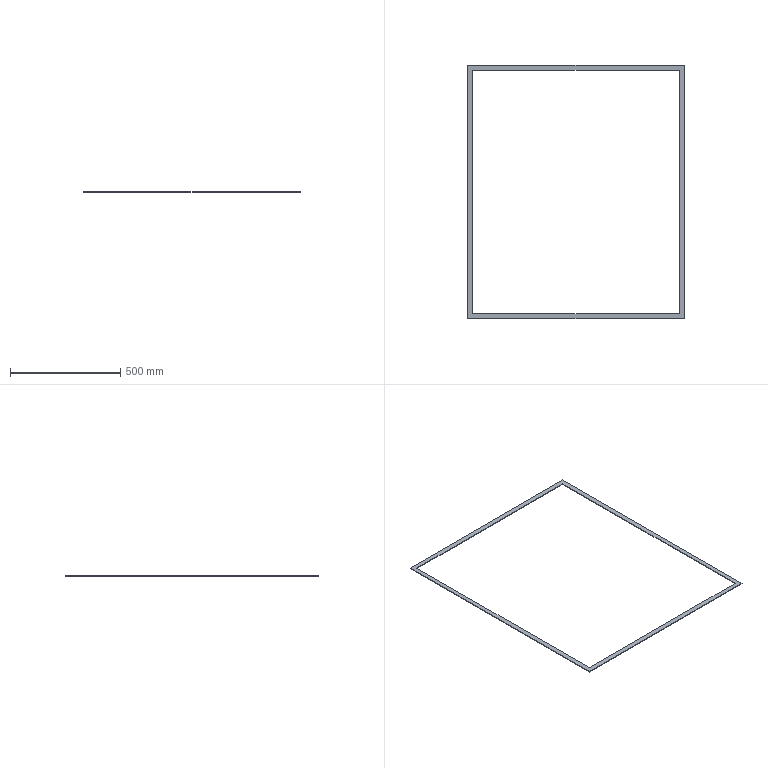Part | STEP file | 750038384 | 1 solid | 10 faces | box 981 x 1150 x 3 mm | volume 275484 mm3 | plane 10
STEP:
#1=CARTESIAN_POINT('',(490.5,-575.,0.));
#2=VERTEX_POINT('',#1);
#3=CARTESIAN_POINT('',(490.5,575.,0.));
#4=VERTEX_POINT('',#3);
#5=CARTESIAN_POINT('',(490.5,0.,0.));
#6=DIRECTION('',(0.,1.,0.));
#7=VECTOR('',#6,1000.);
#8=LINE('',#5,#7);
#9=EDGE_CURVE('',#2,#4,#8,.T.);
#10=ORIENTED_EDGE('',*,*,#9,.F.);
#11=CARTESIAN_POINT('',(-490.5,-575.,0.));
#12=VERTEX_POINT('',#11);
#13=CARTESIAN_POINT('',(0.,-575.,0.));
#14=DIRECTION('',(1.,0.,0.));
#15=VECTOR('',#14,1000.);
#16=LINE('',#13,#15);
#17=EDGE_CURVE('',#12,#2,#16,.T.);
#18=ORIENTED_EDGE('',*,*,#17,.F.);
#19=CARTESIAN_POINT('',(-490.5,575.,0.));
#20=VERTEX_POINT('',#19);
#21=CARTESIAN_POINT('',(-490.5,0.,0.));
#22=DIRECTION('',(0.,-1.,0.));
#23=VECTOR('',#22,1000.);
#24=LINE('',#21,#23);
#25=EDGE_CURVE('',#20,#12,#24,.T.);
#26=ORIENTED_EDGE('',*,*,#25,.F.);
#27=CARTESIAN_POINT('',(0.,575.,0.));
#28=DIRECTION('',(-1.,0.,0.));
#29=VECTOR('',#28,1000.);
#30=LINE('',#27,#29);
#31=EDGE_CURVE('',#4,#20,#30,.T.);
#32=ORIENTED_EDGE('',*,*,#31,.F.);
#33=EDGE_LOOP('',(#10,#18,#26,#32));
#34=FACE_OUTER_BOUND('',#33,.T.);
#35=CARTESIAN_POINT('',(468.5,-553.,0.));
#36=VERTEX_POINT('',#35);
#37=CARTESIAN_POINT('',(-468.5,-553.,0.));
#38=VERTEX_POINT('',#37);
#39=CARTESIAN_POINT('',(0.,-553.,0.));
#40=DIRECTION('',(-1.,0.,0.));
#41=VECTOR('',#40,1000.);
#42=LINE('',#39,#41);
#43=EDGE_CURVE('',#36,#38,#42,.T.);
#44=ORIENTED_EDGE('',*,*,#43,.F.);
#45=CARTESIAN_POINT('',(468.5,553.,0.));
#46=VERTEX_POINT('',#45);
#47=CARTESIAN_POINT('',(468.5,0.,0.));
#48=DIRECTION('',(0.,-1.,0.));
#49=VECTOR('',#48,1000.);
#50=LINE('',#47,#49);
#51=EDGE_CURVE('',#46,#36,#50,.T.);
#52=ORIENTED_EDGE('',*,*,#51,.F.);
#53=CARTESIAN_POINT('',(-468.5,553.,0.));
#54=VERTEX_POINT('',#53);
#55=CARTESIAN_POINT('',(0.,553.,0.));
#56=DIRECTION('',(1.,0.,0.));
#57=VECTOR('',#56,1000.);
#58=LINE('',#55,#57);
#59=EDGE_CURVE('',#54,#46,#58,.T.);
#60=ORIENTED_EDGE('',*,*,#59,.F.);
#61=CARTESIAN_POINT('',(-468.5,0.,0.));
#62=DIRECTION('',(0.,1.,0.));
#63=VECTOR('',#62,1000.);
#64=LINE('',#61,#63);
#65=EDGE_CURVE('',#38,#54,#64,.T.);
#66=ORIENTED_EDGE('',*,*,#65,.F.);
#67=EDGE_LOOP('',(#44,#52,#60,#66));
#68=FACE_BOUND('',#67,.T.);
#69=CARTESIAN_POINT('',(0.,0.,0.));
#70=DIRECTION('',(0.,0.,1.));
#71=DIRECTION('',(1.,0.,0.));
#72=AXIS2_PLACEMENT_3D('',#69,#70,#71);
#73=PLANE('',#72);
#74=ADVANCED_FACE('',(#34,#68),#73,.F.);
#75=CARTESIAN_POINT('',(-490.5,575.,3.));
#76=VERTEX_POINT('',#75);
#77=CARTESIAN_POINT('',(-490.5,575.,3.));
#78=DIRECTION('',(0.,0.,-1.));
#79=VECTOR('',#78,1000.);
#80=LINE('',#77,#79);
#81=EDGE_CURVE('',#76,#20,#80,.T.);
#82=ORIENTED_EDGE('',*,*,#81,.F.);
#83=CARTESIAN_POINT('',(490.5,575.,3.));
#84=VERTEX_POINT('',#83);
#85=CARTESIAN_POINT('',(490.5,575.,3.));
#86=DIRECTION('',(-1.,0.,0.));
#87=VECTOR('',#86,1000.);
#88=LINE('',#85,#87);
#89=EDGE_CURVE('',#84,#76,#88,.T.);
#90=ORIENTED_EDGE('',*,*,#89,.F.);
#91=CARTESIAN_POINT('',(490.5,575.,3.));
#92=DIRECTION('',(0.,0.,1.));
#93=VECTOR('',#92,1000.);
#94=LINE('',#91,#93);
#95=EDGE_CURVE('',#4,#84,#94,.T.);
#96=ORIENTED_EDGE('',*,*,#95,.F.);
#97=ORIENTED_EDGE('',*,*,#31,.T.);
#98=EDGE_LOOP('',(#82,#90,#96,#97));
#99=FACE_OUTER_BOUND('',#98,.T.);
#100=CARTESIAN_POINT('',(490.5,575.,3.));
#101=DIRECTION('',(0.,-1.,0.));
#102=DIRECTION('',(0.,0.,-1.));
#103=AXIS2_PLACEMENT_3D('',#100,#101,#102);
#104=PLANE('',#103);
#105=ADVANCED_FACE('',(#99),#104,.F.);
#106=ORIENTED_EDGE('',*,*,#95,.T.);
#107=CARTESIAN_POINT('',(490.5,-575.,3.));
#108=VERTEX_POINT('',#107);
#109=CARTESIAN_POINT('',(490.5,-575.,3.));
#110=DIRECTION('',(0.,1.,0.));
#111=VECTOR('',#110,1000.);
#112=LINE('',#109,#111);
#113=EDGE_CURVE('',#108,#84,#112,.T.);
#114=ORIENTED_EDGE('',*,*,#113,.F.);
#115=CARTESIAN_POINT('',(490.5,-575.,3.));
#116=DIRECTION('',(0.,0.,1.));
#117=VECTOR('',#116,1000.);
#118=LINE('',#115,#117);
#119=EDGE_CURVE('',#2,#108,#118,.T.);
#120=ORIENTED_EDGE('',*,*,#119,.F.);
#121=ORIENTED_EDGE('',*,*,#9,.T.);
#122=EDGE_LOOP('',(#106,#114,#120,#121));
#123=FACE_OUTER_BOUND('',#122,.T.);
#124=CARTESIAN_POINT('',(490.5,-575.,3.));
#125=DIRECTION('',(-1.,0.,0.));
#126=DIRECTION('',(0.,-1.,0.));
#127=AXIS2_PLACEMENT_3D('',#124,#125,#126);
#128=PLANE('',#127);
#129=ADVANCED_FACE('',(#123),#128,.F.);
#130=ORIENTED_EDGE('',*,*,#119,.T.);
#131=CARTESIAN_POINT('',(-490.5,-575.,3.));
#132=VERTEX_POINT('',#131);
#133=CARTESIAN_POINT('',(-490.5,-575.,3.));
#134=DIRECTION('',(1.,0.,0.));
#135=VECTOR('',#134,1000.);
#136=LINE('',#133,#135);
#137=EDGE_CURVE('',#132,#108,#136,.T.);
#138=ORIENTED_EDGE('',*,*,#137,.F.);
#139=CARTESIAN_POINT('',(-490.5,-575.,3.));
#140=DIRECTION('',(0.,0.,1.));
#141=VECTOR('',#140,1000.);
#142=LINE('',#139,#141);
#143=EDGE_CURVE('',#12,#132,#142,.T.);
#144=ORIENTED_EDGE('',*,*,#143,.F.);
#145=ORIENTED_EDGE('',*,*,#17,.T.);
#146=EDGE_LOOP('',(#130,#138,#144,#145));
#147=FACE_OUTER_BOUND('',#146,.T.);
#148=CARTESIAN_POINT('',(-490.5,-575.,3.));
#149=DIRECTION('',(0.,1.,0.));
#150=DIRECTION('',(0.,0.,1.));
#151=AXIS2_PLACEMENT_3D('',#148,#149,#150);
#152=PLANE('',#151);
#153=ADVANCED_FACE('',(#147),#152,.F.);
#154=ORIENTED_EDGE('',*,*,#143,.T.);
#155=CARTESIAN_POINT('',(-490.5,575.,3.));
#156=DIRECTION('',(0.,-1.,0.));
#157=VECTOR('',#156,1000.);
#158=LINE('',#155,#157);
#159=EDGE_CURVE('',#76,#132,#158,.T.);
#160=ORIENTED_EDGE('',*,*,#159,.F.);
#161=ORIENTED_EDGE('',*,*,#81,.T.);
#162=ORIENTED_EDGE('',*,*,#25,.T.);
#163=EDGE_LOOP('',(#154,#160,#161,#162));
#164=FACE_OUTER_BOUND('',#163,.T.);
#165=CARTESIAN_POINT('',(-490.5,575.,3.));
#166=DIRECTION('',(1.,0.,0.));
#167=DIRECTION('',(0.,1.,0.));
#168=AXIS2_PLACEMENT_3D('',#165,#166,#167);
#169=PLANE('',#168);
#170=ADVANCED_FACE('',(#164),#169,.F.);
#171=CARTESIAN_POINT('',(-468.5,553.,3.));
#172=VERTEX_POINT('',#171);
#173=CARTESIAN_POINT('',(-468.5,-553.,3.));
#174=VERTEX_POINT('',#173);
#175=CARTESIAN_POINT('',(-468.5,553.,3.));
#176=DIRECTION('',(0.,-1.,0.));
#177=VECTOR('',#176,1000.);
#178=LINE('',#175,#177);
#179=EDGE_CURVE('',#172,#174,#178,.T.);
#180=ORIENTED_EDGE('',*,*,#179,.T.);
#181=CARTESIAN_POINT('',(-468.5,-553.,3.));
#182=DIRECTION('',(0.,0.,-1.));
#183=VECTOR('',#182,1000.);
#184=LINE('',#181,#183);
#185=EDGE_CURVE('',#174,#38,#184,.T.);
#186=ORIENTED_EDGE('',*,*,#185,.T.);
#187=ORIENTED_EDGE('',*,*,#65,.T.);
#188=CARTESIAN_POINT('',(-468.5,553.,3.));
#189=DIRECTION('',(0.,0.,1.));
#190=VECTOR('',#189,1000.);
#191=LINE('',#188,#190);
#192=EDGE_CURVE('',#54,#172,#191,.T.);
#193=ORIENTED_EDGE('',*,*,#192,.T.);
#194=EDGE_LOOP('',(#180,#186,#187,#193));
#195=FACE_OUTER_BOUND('',#194,.T.);
#196=CARTESIAN_POINT('',(-468.5,553.,3.));
#197=DIRECTION('',(1.,0.,0.));
#198=DIRECTION('',(0.,1.,0.));
#199=AXIS2_PLACEMENT_3D('',#196,#197,#198);
#200=PLANE('',#199);
#201=ADVANCED_FACE('',(#195),#200,.T.);
#202=CARTESIAN_POINT('',(468.5,-553.,3.));
#203=VERTEX_POINT('',#202);
#204=CARTESIAN_POINT('',(-468.5,-553.,3.));
#205=DIRECTION('',(1.,0.,0.));
#206=VECTOR('',#205,1000.);
#207=LINE('',#204,#206);
#208=EDGE_CURVE('',#174,#203,#207,.T.);
#209=ORIENTED_EDGE('',*,*,#208,.T.);
#210=CARTESIAN_POINT('',(468.5,-553.,3.));
#211=DIRECTION('',(0.,0.,-1.));
#212=VECTOR('',#211,1000.);
#213=LINE('',#210,#212);
#214=EDGE_CURVE('',#203,#36,#213,.T.);
#215=ORIENTED_EDGE('',*,*,#214,.T.);
#216=ORIENTED_EDGE('',*,*,#43,.T.);
#217=ORIENTED_EDGE('',*,*,#185,.F.);
#218=EDGE_LOOP('',(#209,#215,#216,#217));
#219=FACE_OUTER_BOUND('',#218,.T.);
#220=CARTESIAN_POINT('',(-468.5,-553.,3.));
#221=DIRECTION('',(0.,1.,0.));
#222=DIRECTION('',(0.,0.,1.));
#223=AXIS2_PLACEMENT_3D('',#220,#221,#222);
#224=PLANE('',#223);
#225=ADVANCED_FACE('',(#219),#224,.T.);
#226=CARTESIAN_POINT('',(468.5,553.,3.));
#227=VERTEX_POINT('',#226);
#228=CARTESIAN_POINT('',(468.5,-553.,3.));
#229=DIRECTION('',(0.,1.,0.));
#230=VECTOR('',#229,1000.);
#231=LINE('',#228,#230);
#232=EDGE_CURVE('',#203,#227,#231,.T.);
#233=ORIENTED_EDGE('',*,*,#232,.T.);
#234=CARTESIAN_POINT('',(468.5,553.,3.));
#235=DIRECTION('',(0.,0.,-1.));
#236=VECTOR('',#235,1000.);
#237=LINE('',#234,#236);
#238=EDGE_CURVE('',#227,#46,#237,.T.);
#239=ORIENTED_EDGE('',*,*,#238,.T.);
#240=ORIENTED_EDGE('',*,*,#51,.T.);
#241=ORIENTED_EDGE('',*,*,#214,.F.);
#242=EDGE_LOOP('',(#233,#239,#240,#241));
#243=FACE_OUTER_BOUND('',#242,.T.);
#244=CARTESIAN_POINT('',(468.5,-553.,3.));
#245=DIRECTION('',(-1.,0.,0.));
#246=DIRECTION('',(0.,-1.,0.));
#247=AXIS2_PLACEMENT_3D('',#244,#245,#246);
#248=PLANE('',#247);
#249=ADVANCED_FACE('',(#243),#248,.T.);
#250=CARTESIAN_POINT('',(468.5,553.,3.));
#251=DIRECTION('',(-1.,0.,0.));
#252=VECTOR('',#251,1000.);
#253=LINE('',#250,#252);
#254=EDGE_CURVE('',#227,#172,#253,.T.);
#255=ORIENTED_EDGE('',*,*,#254,.T.);
#256=ORIENTED_EDGE('',*,*,#192,.F.);
#257=ORIENTED_EDGE('',*,*,#59,.T.);
#258=ORIENTED_EDGE('',*,*,#238,.F.);
#259=EDGE_LOOP('',(#255,#256,#257,#258));
#260=FACE_OUTER_BOUND('',#259,.T.);
#261=CARTESIAN_POINT('',(468.5,553.,3.));
#262=DIRECTION('',(0.,-1.,0.));
#263=DIRECTION('',(0.,0.,-1.));
#264=AXIS2_PLACEMENT_3D('',#261,#262,#263);
#265=PLANE('',#264);
#266=ADVANCED_FACE('',(#260),#265,.T.);
#267=ORIENTED_EDGE('',*,*,#137,.T.);
#268=ORIENTED_EDGE('',*,*,#113,.T.);
#269=ORIENTED_EDGE('',*,*,#89,.T.);
#270=ORIENTED_EDGE('',*,*,#159,.T.);
#271=EDGE_LOOP('',(#267,#268,#269,#270));
#272=FACE_OUTER_BOUND('',#271,.T.);
#273=ORIENTED_EDGE('',*,*,#232,.F.);
#274=ORIENTED_EDGE('',*,*,#208,.F.);
#275=ORIENTED_EDGE('',*,*,#179,.F.);
#276=ORIENTED_EDGE('',*,*,#254,.F.);
#277=EDGE_LOOP('',(#273,#274,#275,#276));
#278=FACE_BOUND('',#277,.T.);
#279=CARTESIAN_POINT('',(0.,0.,3.));
#280=DIRECTION('',(0.,0.,1.));
#281=DIRECTION('',(1.,0.,0.));
#282=AXIS2_PLACEMENT_3D('',#279,#280,#281);
#283=PLANE('',#282);
#284=ADVANCED_FACE('',(#272,#278),#283,.T.);
#285=CLOSED_SHELL('',(#74,#105,#129,#153,#170,#201,#225,#249,#266,#284));
#286=MANIFOLD_SOLID_BREP('',#285);
#287=CARTESIAN_POINT('',(0.,0.,0.));
#288=DIRECTION('',(0.,0.,1.));
#289=DIRECTION('',(1.,0.,0.));
#290=AXIS2_PLACEMENT_3D('',#287,#288,#289);
#291=(LENGTH_UNIT()NAMED_UNIT(*)SI_UNIT(.MILLI.,.METRE.));
#292=UNCERTAINTY_MEASURE_WITH_UNIT(LENGTH_MEASURE(0.00001),#291,'','');
#293=(NAMED_UNIT(*)PLANE_ANGLE_UNIT()SI_UNIT($,.RADIAN.));
#294=(NAMED_UNIT(*)SI_UNIT($,.STERADIAN.)SOLID_ANGLE_UNIT());
#295=(GEOMETRIC_REPRESENTATION_CONTEXT(3)GLOBAL_UNCERTAINTY_ASSIGNED_CONTEXT((#292))GLOBAL_UNIT_ASSIGNED_CONTEXT((#291,#293,#294))REPRESENTATION_CONTEXT('',''));
#296=ADVANCED_BREP_SHAPE_REPRESENTATION('',(#286,#290),#295);